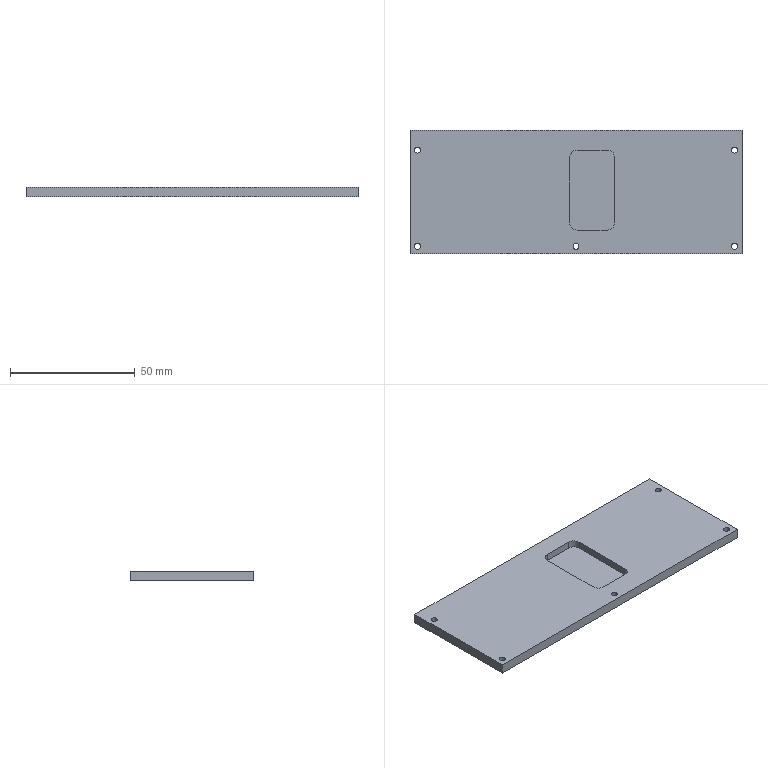NC program | NX | posted with a generic post | part box 133 x 49.5 x 4 mm
Whole program:
N10 G17 G21 G94 G90
(HOLE_MILLING , TOOL : D3)
N12 T03 M6
N14 G54
N16 G17 G0 G90 X-63.5 Y16.75 S9500 M3
N18 G43 Z30. H3
N20 Z0.5
N22 G94 G3 X-63.75 Y17. R0.25 F1250.
N24 X-64. Y16.75 R0.25
N26 X-64. Y16.75 Z0.35 I0.5 J0.
N28 X-64. Y16.75 Z0.2 I0.5 J0.
N30 X-64. Y16.75 Z0.05 I0.5 J0.
N32 X-64. Y16.75 Z-0.1 I0.5 J0.
N34 X-64. Y16.75 Z-0.25 I0.5 J0.
N36 X-64. Y16.75 Z-0.4 I0.5 J0.
N38 X-64. Y16.75 Z-0.55 I0.5 J0.
N40 X-64. Y16.75 Z-0.7 I0.5 J0.
N42 X-64. Y16.75 Z-0.85 I0.5 J0.
N44 X-64. Y16.75 Z-1. I0.5 J0.
N46 X-64. Y16.75 Z-1.15 I0.5 J0.
N48 X-64. Y16.75 Z-1.3 I0.5 J0.
N50 X-64. Y16.75 Z-1.45 I0.5 J0.
N52 X-64. Y16.75 Z-1.6 I0.5 J0.
N54 X-64. Y16.75 Z-1.75 I0.5 J0.
N56 X-64. Y16.75 Z-1.9 I0.5 J0.
N58 X-64. Y16.75 Z-2.05 I0.5 J0.
N60 X-64. Y16.75 Z-2.2 I0.5 J0.
N62 X-63.25 Y17.183 Z-2.3 R-0.5
N64 X-63.933 Y17. R0.5
N66 X-63.25 Y17.183 R-0.5
N68 X-63.592 Y17.092 R0.25
N70 X-63.5 Y16.75 R0.25
N72 G0 Z30.
N74 Y-21.75
N76 Z0.5
N78 G3 X-63.75 Y-21.5 R0.25
N80 X-64. Y-21.75 R0.25
N82 X-64. Y-21.75 Z0.35 I0.5 J0.
N84 X-64. Y-21.75 Z0.2 I0.5 J0.
N86 X-64. Y-21.75 Z0.05 I0.5 J0.
N88 X-64. Y-21.75 Z-0.1 I0.5 J0.
N90 X-64. Y-21.75 Z-0.25 I0.5 J0.
N92 X-64. Y-21.75 Z-0.4 I0.5 J0.
N94 X-64. Y-21.75 Z-0.55 I0.5 J0.
N96 X-64. Y-21.75 Z-0.7 I0.5 J0.
N98 X-64. Y-21.75 Z-0.85 I0.5 J0.
N100 X-64. Y-21.75 Z-1. I0.5 J0.
N102 X-64. Y-21.75 Z-1.15 I0.5 J0.
N104 X-64. Y-21.75 Z-1.3 I0.5 J0.
N106 X-64. Y-21.75 Z-1.45 I0.5 J0.
N108 X-64. Y-21.75 Z-1.6 I0.5 J0.
N110 X-64. Y-21.75 Z-1.75 I0.5 J0.
N112 X-64. Y-21.75 Z-1.9 I0.5 J0.
N114 X-64. Y-21.75 Z-2.05 I0.5 J0.
N116 X-64. Y-21.75 Z-2.2 I0.5 J0.
N118 X-63.25 Y-21.317 Z-2.3 R-0.5
N120 X-63.933 Y-21.5 R0.5
N122 X-63.25 Y-21.317 R-0.5
N124 X-63.592 Y-21.408 R0.25
N126 X-63.5 Y-21.75 R0.25
N128 G0 Z30.
N130 X0.
N132 Z0.5
N134 G3 X-0.25 Y-21.5 R0.25
N136 X-0.5 Y-21.75 R0.25
N138 X-0.5 Y-21.75 Z0.35 I0.5 J0.
N140 X-0.5 Y-21.75 Z0.2 I0.5 J0.
N142 X-0.5 Y-21.75 Z0.05 I0.5 J0.
N144 X-0.5 Y-21.75 Z-0.1 I0.5 J0.
N146 X-0.5 Y-21.75 Z-0.25 I0.5 J0.
N148 X-0.5 Y-21.75 Z-0.4 I0.5 J0.
N150 X-0.5 Y-21.75 Z-0.55 I0.5 J0.
N152 X-0.5 Y-21.75 Z-0.7 I0.5 J0.
N154 X-0.5 Y-21.75 Z-0.85 I0.5 J0.
N156 X-0.5 Y-21.75 Z-1. I0.5 J0.
N158 X-0.5 Y-21.75 Z-1.15 I0.5 J0.
N160 X-0.5 Y-21.75 Z-1.3 I0.5 J0.
N162 X-0.5 Y-21.75 Z-1.45 I0.5 J0.
N164 X-0.5 Y-21.75 Z-1.6 I0.5 J0.
N166 X-0.5 Y-21.75 Z-1.75 I0.5 J0.
N168 X-0.5 Y-21.75 Z-1.9 I0.5 J0.
N170 X-0.5 Y-21.75 Z-2.05 I0.5 J0.
N172 X-0.5 Y-21.75 Z-2.2 I0.5 J0.
N174 X0.25 Y-21.317 Z-2.3 R-0.5
N176 X-0.433 Y-21.5 R0.5
N178 X0.25 Y-21.317 R-0.5
N180 X-0.092 Y-21.408 R0.25
N182 X0. Y-21.75 R0.25
N184 G0 Z30.
N186 X63.5 Y16.75
N188 Z0.5
N190 G3 X63.25 Y17. R0.25
N192 X63. Y16.75 R0.25
N194 X63. Y16.75 Z0.35 I0.5 J0.
N196 X63. Y16.75 Z0.2 I0.5 J0.
N198 X63. Y16.75 Z0.05 I0.5 J0.
N200 X63. Y16.75 Z-0.1 I0.5 J0.
N202 X63. Y16.75 Z-0.25 I0.5 J0.
N204 X63. Y16.75 Z-0.4 I0.5 J0.
N206 X63. Y16.75 Z-0.55 I0.5 J0.
N208 X63. Y16.75 Z-0.7 I0.5 J0.
N210 X63. Y16.75 Z-0.85 I0.5 J0.
N212 X63. Y16.75 Z-1. I0.5 J0.
N214 X63. Y16.75 Z-1.15 I0.5 J0.
N216 X63. Y16.75 Z-1.3 I0.5 J0.
N218 X63. Y16.75 Z-1.45 I0.5 J0.
N220 X63. Y16.75 Z-1.6 I0.5 J0.
N222 X63. Y16.75 Z-1.75 I0.5 J0.
N224 X63. Y16.75 Z-1.9 I0.5 J0.
N226 X63. Y16.75 Z-2.05 I0.5 J0.
N228 X63. Y16.75 Z-2.2 I0.5 J0.
N230 X63.75 Y17.183 Z-2.3 R-0.5
N232 X63.067 Y17. R0.5
N234 X63.75 Y17.183 R-0.5
N236 X63.408 Y17.092 R0.25
N238 X63.5 Y16.75 R0.25
N240 G0 Z30.
N242 Y-21.75
N244 Z0.5
N246 G3 X63.25 Y-21.5 R0.25
N248 X63. Y-21.75 R0.25
N250 X63. Y-21.75 Z0.35 I0.5 J0.
N252 X63. Y-21.75 Z0.2 I0.5 J0.
N254 X63. Y-21.75 Z0.05 I0.5 J0.
N256 X63. Y-21.75 Z-0.1 I0.5 J0.
N258 X63. Y-21.75 Z-0.25 I0.5 J0.
N260 X63. Y-21.75 Z-0.4 I0.5 J0.
N262 X63. Y-21.75 Z-0.55 I0.5 J0.
N264 X63. Y-21.75 Z-0.7 I0.5 J0.
N266 X63. Y-21.75 Z-0.85 I0.5 J0.
N268 X63. Y-21.75 Z-1. I0.5 J0.
N270 X63. Y-21.75 Z-1.15 I0.5 J0.
N272 X63. Y-21.75 Z-1.3 I0.5 J0.
N274 X63. Y-21.75 Z-1.45 I0.5 J0.
N276 X63. Y-21.75 Z-1.6 I0.5 J0.
N278 X63. Y-21.75 Z-1.75 I0.5 J0.
N280 X63. Y-21.75 Z-1.9 I0.5 J0.
N282 X63. Y-21.75 Z-2.05 I0.5 J0.
N284 X63. Y-21.75 Z-2.2 I0.5 J0.
N286 X63.75 Y-21.317 Z-2.3 R-0.5
N288 X63.067 Y-21.5 R0.5
N290 X63.75 Y-21.317 R-0.5
N292 X63.408 Y-21.408 R0.25
N294 X63.5 Y-21.75 R0.25
N296 G0 Z30.
N298 M5
(ZLEVEL_PROFILE_1_COPY_COPY , TOOL : D6A45)
N300 T07 M6
N302 G54
N304 G17 G0 G90 X-64.549 Y16.75 S9500 M3
N306 G43 Z30. H7
N308 Z2.
N310 G94 G1 Z-1. F1250.
N312 Y16.746
N314 G3 X-63.496 Y15.701 R1.049
N316 X-64.549 Y16.75 R-1.049
N318 X-64.249 Y16.23 R0.6
N320 G1 Z1.
N322 G0 Z30.
N324 X64.549 Y-21.75
N326 Z2.
N328 G1 Z-1.
N330 Y-21.742
N332 G3 X63.492 Y-20.701 R1.049
N334 X64.549 Y-21.75 R-1.049
N336 X64.249 Y-21.23 R0.6
N338 G1 Z1.
N340 G0 Z30.
N342 X0. Y-22.799
N344 Z2.
N346 G1 Z-1.
N348 G3 X1.049 Y-21.75 R1.049
N350 X0. Y-22.799 R-1.049
N352 X0.52 Y-22.499 R0.6
N354 G1 Z1.
N356 G0 Z30.
N358 X-64.549 Y-21.75
N360 Z2.
N362 G1 Z-1.
N364 G3 X-63.5 Y-22.799 R1.049
N366 X-64.549 Y-21.75 R-1.049
N368 X-64.249 Y-22.27 R0.6
N370 G1 Z1.
N372 G0 Z30.
N374 X64.549 Y16.75
N376 Z2.
N378 G1 Z-1.
N380 G3 X63.5 Y17.799 R1.049
N382 X64.549 Y16.75 R-1.049
N384 X64.249 Y17.27 R0.6
N386 G1 Z1.
N388 G0 Z30.
N390 X-67.418 Y26.686
N392 Z1.
N394 G1 Z-1.
N396 X-67.022 Y26.001
N398 G3 X-66.503 Y25.701 R0.6
N400 G1 X66.503
N402 G2 X67.451 Y24.753 R0.977
N404 G1 Y-24.753
N406 G2 X66.503 Y-25.701 R0.977
N408 G1 X-66.503
N410 G2 X-67.451 Y-24.753 R0.977
N412 G1 Y24.753
N414 G2 X-66.503 Y25.701 R0.977
N416 G3 X-65.992 Y26.016 R0.6
N418 G1 X-65.514 Y26.901
N420 Z1.
N422 G0 Z30.
N424 M5
N426 M2